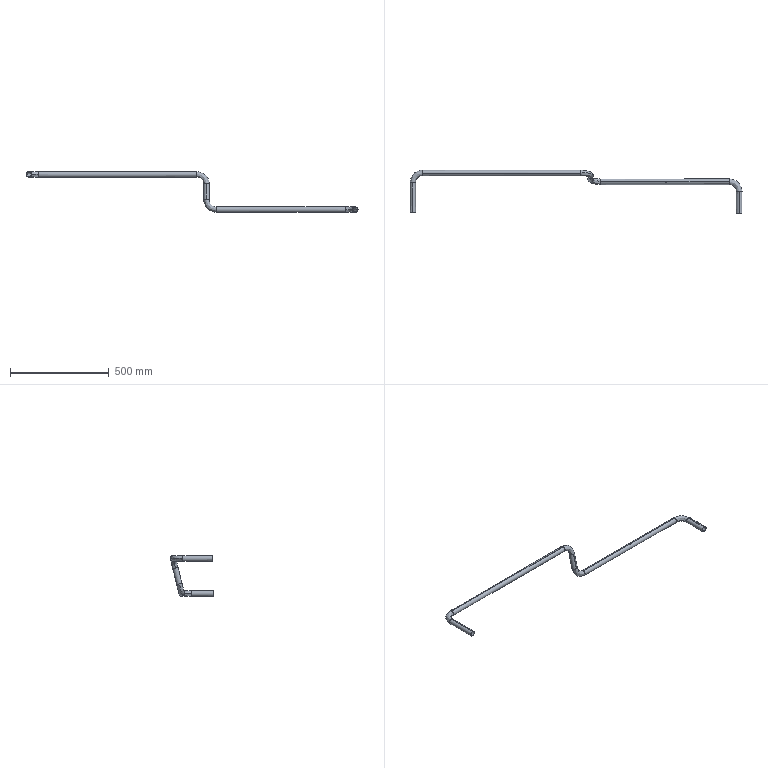Part | STEP file | copper tube 4_default_machined_ | 1 solid | 40 faces | box 1681 x 220 x 205.42 mm | volume 263812 mm3 | cylinder 22 | spline 16 | plane 2 | commonest cylinder face diameters 25 x10 28 x10 6.5 x2